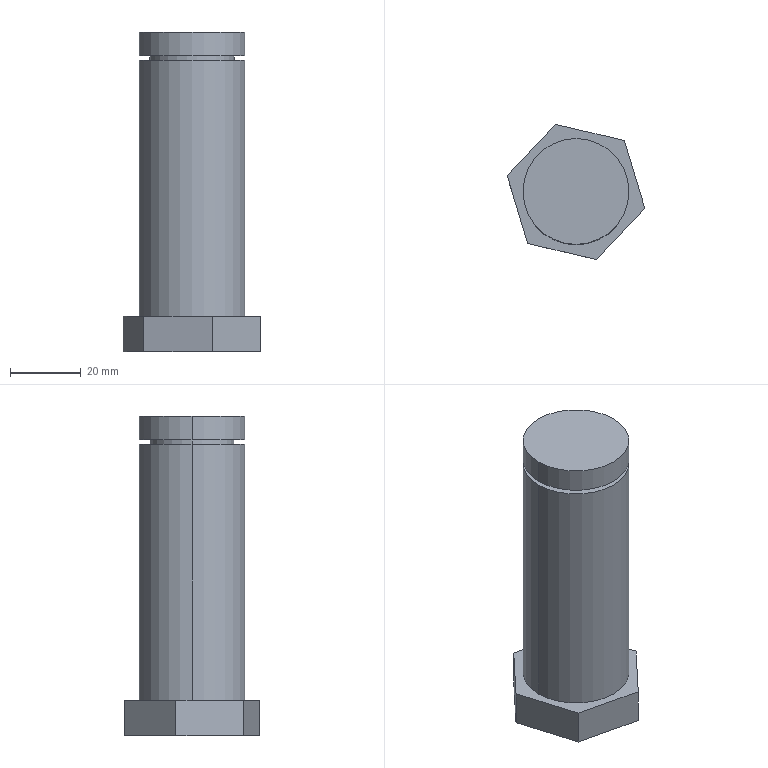Part | STEP file | 1 solid | 17 faces | box 38.947 x 38.288 x 90.5 mm | volume 66959 mm3 | plane 11 | cylinder 6 | commonest cylinder face diameters 30 x4 23.9 x2
STEP:
#1=CARTESIAN_POINT('',(0.,0.,0.));
#2=DIRECTION('',(0.,0.,1.));
#3=DIRECTION('',(1.,0.,0.));
#4=AXIS2_PLACEMENT_3D('',#1,#2,#3);
#5=CARTESIAN_POINT('',(-5.789,19.144,0.));
#6=VERTEX_POINT('',#5);
#7=CARTESIAN_POINT('',(13.684,14.585,0.));
#8=VERTEX_POINT('',#7);
#9=CARTESIAN_POINT('',(-5.789,19.144,0.));
#10=DIRECTION('',(0.9737,-0.2279,0.));
#11=VECTOR('',#10,1.);
#12=LINE('',#9,#11);
#13=CARTESIAN_POINT('',(0.,0.,0.));
#14=DIRECTION('',(0.,0.,1.));
#15=DIRECTION('',(1.,0.,0.));
#16=AXIS2_PLACEMENT_3D('',#13,#14,#15);
#17=PLANE('',#16);
#18=CARTESIAN_POINT('',(-5.789,19.144));
#19=DIRECTION('',(0.9737,-0.2279));
#20=VECTOR('',#19,1.);
#21=LINE('',#18,#20);
#22=(GEOMETRIC_REPRESENTATION_CONTEXT(2)PARAMETRIC_REPRESENTATION_CONTEXT()REPRESENTATION_CONTEXT('',''));
#23=DEFINITIONAL_REPRESENTATION('',(#21),#22);
#24=PCURVE('',#17,#23);
#25=CARTESIAN_POINT('',(-5.789,19.144,80.5));
#26=DIRECTION('',(0.2279,0.9737,0.));
#27=DIRECTION('',(0.,0.,-1.));
#28=AXIS2_PLACEMENT_3D('',#25,#26,#27);
#29=PLANE('',#28);
#30=CARTESIAN_POINT('',(80.5,0.));
#31=DIRECTION('',(0.,-1.));
#32=VECTOR('',#31,1.);
#33=LINE('',#30,#32);
#34=(GEOMETRIC_REPRESENTATION_CONTEXT(2)PARAMETRIC_REPRESENTATION_CONTEXT()REPRESENTATION_CONTEXT('',''));
#35=DEFINITIONAL_REPRESENTATION('',(#33),#34);
#36=PCURVE('',#29,#35);
#37=SURFACE_CURVE('',#12,(#24,#36),.PCURVE_S1.);
#38=EDGE_CURVE('',#6,#8,#37,.T.);
#39=ORIENTED_EDGE('',*,*,#38,.T.);
#40=CARTESIAN_POINT('',(19.474,-4.558,0.));
#41=VERTEX_POINT('',#40);
#42=CARTESIAN_POINT('',(13.684,14.585,0.));
#43=DIRECTION('',(0.2895,-0.9572,0.));
#44=VECTOR('',#43,1.);
#45=LINE('',#42,#44);
#46=CARTESIAN_POINT('',(13.684,14.585));
#47=DIRECTION('',(0.2895,-0.9572));
#48=VECTOR('',#47,1.);
#49=LINE('',#46,#48);
#50=(GEOMETRIC_REPRESENTATION_CONTEXT(2)PARAMETRIC_REPRESENTATION_CONTEXT()REPRESENTATION_CONTEXT('',''));
#51=DEFINITIONAL_REPRESENTATION('',(#49),#50);
#52=PCURVE('',#17,#51);
#53=CARTESIAN_POINT('',(13.684,14.585,80.5));
#54=DIRECTION('',(0.9572,0.2895,0.));
#55=DIRECTION('',(0.,0.,-1.));
#56=AXIS2_PLACEMENT_3D('',#53,#54,#55);
#57=PLANE('',#56);
#58=CARTESIAN_POINT('',(80.5,0.));
#59=DIRECTION('',(0.,-1.));
#60=VECTOR('',#59,1.);
#61=LINE('',#58,#60);
#62=(GEOMETRIC_REPRESENTATION_CONTEXT(2)PARAMETRIC_REPRESENTATION_CONTEXT()REPRESENTATION_CONTEXT('',''));
#63=DEFINITIONAL_REPRESENTATION('',(#61),#62);
#64=PCURVE('',#57,#63);
#65=SURFACE_CURVE('',#45,(#52,#64),.PCURVE_S1.);
#66=EDGE_CURVE('',#8,#41,#65,.T.);
#67=ORIENTED_EDGE('',*,*,#66,.T.);
#68=CARTESIAN_POINT('',(5.789,-19.144,0.));
#69=VERTEX_POINT('',#68);
#70=CARTESIAN_POINT('',(19.474,-4.558,0.));
#71=DIRECTION('',(-0.6842,-0.7293,0.));
#72=VECTOR('',#71,1.);
#73=LINE('',#70,#72);
#74=CARTESIAN_POINT('',(19.474,-4.558));
#75=DIRECTION('',(-0.6842,-0.7293));
#76=VECTOR('',#75,1.);
#77=LINE('',#74,#76);
#78=(GEOMETRIC_REPRESENTATION_CONTEXT(2)PARAMETRIC_REPRESENTATION_CONTEXT()REPRESENTATION_CONTEXT('',''));
#79=DEFINITIONAL_REPRESENTATION('',(#77),#78);
#80=PCURVE('',#17,#79);
#81=CARTESIAN_POINT('',(19.474,-4.558,80.5));
#82=DIRECTION('',(0.7293,-0.6842,0.));
#83=DIRECTION('',(0.,0.,-1.));
#84=AXIS2_PLACEMENT_3D('',#81,#82,#83);
#85=PLANE('',#84);
#86=CARTESIAN_POINT('',(80.5,0.));
#87=DIRECTION('',(0.,-1.));
#88=VECTOR('',#87,1.);
#89=LINE('',#86,#88);
#90=(GEOMETRIC_REPRESENTATION_CONTEXT(2)PARAMETRIC_REPRESENTATION_CONTEXT()REPRESENTATION_CONTEXT('',''));
#91=DEFINITIONAL_REPRESENTATION('',(#89),#90);
#92=PCURVE('',#85,#91);
#93=SURFACE_CURVE('',#73,(#80,#92),.PCURVE_S1.);
#94=EDGE_CURVE('',#41,#69,#93,.T.);
#95=ORIENTED_EDGE('',*,*,#94,.T.);
#96=CARTESIAN_POINT('',(-13.684,-14.585,0.));
#97=VERTEX_POINT('',#96);
#98=CARTESIAN_POINT('',(5.789,-19.144,0.));
#99=DIRECTION('',(-0.9737,0.2279,0.));
#100=VECTOR('',#99,1.);
#101=LINE('',#98,#100);
#102=CARTESIAN_POINT('',(5.789,-19.144));
#103=DIRECTION('',(-0.9737,0.2279));
#104=VECTOR('',#103,1.);
#105=LINE('',#102,#104);
#106=(GEOMETRIC_REPRESENTATION_CONTEXT(2)PARAMETRIC_REPRESENTATION_CONTEXT()REPRESENTATION_CONTEXT('',''));
#107=DEFINITIONAL_REPRESENTATION('',(#105),#106);
#108=PCURVE('',#17,#107);
#109=CARTESIAN_POINT('',(5.789,-19.144,80.5));
#110=DIRECTION('',(-0.2279,-0.9737,0.));
#111=DIRECTION('',(-0.9737,0.2279,0.));
#112=AXIS2_PLACEMENT_3D('',#109,#110,#111);
#113=PLANE('',#112);
#114=CARTESIAN_POINT('',(0.,80.5));
#115=DIRECTION('',(1.,0.));
#116=VECTOR('',#115,1.);
#117=LINE('',#114,#116);
#118=(GEOMETRIC_REPRESENTATION_CONTEXT(2)PARAMETRIC_REPRESENTATION_CONTEXT()REPRESENTATION_CONTEXT('',''));
#119=DEFINITIONAL_REPRESENTATION('',(#117),#118);
#120=PCURVE('',#113,#119);
#121=SURFACE_CURVE('',#101,(#108,#120),.PCURVE_S1.);
#122=EDGE_CURVE('',#69,#97,#121,.T.);
#123=ORIENTED_EDGE('',*,*,#122,.T.);
#124=CARTESIAN_POINT('',(-19.474,4.558,0.));
#125=VERTEX_POINT('',#124);
#126=CARTESIAN_POINT('',(-13.684,-14.585,0.));
#127=DIRECTION('',(-0.2895,0.9572,0.));
#128=VECTOR('',#127,1.);
#129=LINE('',#126,#128);
#130=CARTESIAN_POINT('',(-13.684,-14.585));
#131=DIRECTION('',(-0.2895,0.9572));
#132=VECTOR('',#131,1.);
#133=LINE('',#130,#132);
#134=(GEOMETRIC_REPRESENTATION_CONTEXT(2)PARAMETRIC_REPRESENTATION_CONTEXT()REPRESENTATION_CONTEXT('',''));
#135=DEFINITIONAL_REPRESENTATION('',(#133),#134);
#136=PCURVE('',#17,#135);
#137=CARTESIAN_POINT('',(-13.684,-14.585,80.5));
#138=DIRECTION('',(-0.9572,-0.2895,0.));
#139=DIRECTION('',(-0.2895,0.9572,0.));
#140=AXIS2_PLACEMENT_3D('',#137,#138,#139);
#141=PLANE('',#140);
#142=CARTESIAN_POINT('',(0.,80.5));
#143=DIRECTION('',(1.,0.));
#144=VECTOR('',#143,1.);
#145=LINE('',#142,#144);
#146=(GEOMETRIC_REPRESENTATION_CONTEXT(2)PARAMETRIC_REPRESENTATION_CONTEXT()REPRESENTATION_CONTEXT('',''));
#147=DEFINITIONAL_REPRESENTATION('',(#145),#146);
#148=PCURVE('',#141,#147);
#149=SURFACE_CURVE('',#129,(#136,#148),.PCURVE_S1.);
#150=EDGE_CURVE('',#97,#125,#149,.T.);
#151=ORIENTED_EDGE('',*,*,#150,.T.);
#152=CARTESIAN_POINT('',(-19.474,4.558,0.));
#153=DIRECTION('',(0.6842,0.7293,0.));
#154=VECTOR('',#153,1.);
#155=LINE('',#152,#154);
#156=CARTESIAN_POINT('',(-19.474,4.558));
#157=DIRECTION('',(0.6842,0.7293));
#158=VECTOR('',#157,1.);
#159=LINE('',#156,#158);
#160=(GEOMETRIC_REPRESENTATION_CONTEXT(2)PARAMETRIC_REPRESENTATION_CONTEXT()REPRESENTATION_CONTEXT('',''));
#161=DEFINITIONAL_REPRESENTATION('',(#159),#160);
#162=PCURVE('',#17,#161);
#163=CARTESIAN_POINT('',(-19.474,4.558,80.5));
#164=DIRECTION('',(-0.7293,0.6842,0.));
#165=DIRECTION('',(0.,0.,1.));
#166=AXIS2_PLACEMENT_3D('',#163,#164,#165);
#167=PLANE('',#166);
#168=CARTESIAN_POINT('',(-80.5,0.));
#169=DIRECTION('',(0.,1.));
#170=VECTOR('',#169,1.);
#171=LINE('',#168,#170);
#172=(GEOMETRIC_REPRESENTATION_CONTEXT(2)PARAMETRIC_REPRESENTATION_CONTEXT()REPRESENTATION_CONTEXT('',''));
#173=DEFINITIONAL_REPRESENTATION('',(#171),#172);
#174=PCURVE('',#167,#173);
#175=SURFACE_CURVE('',#155,(#162,#174),.PCURVE_S1.);
#176=EDGE_CURVE('',#125,#6,#175,.T.);
#177=ORIENTED_EDGE('',*,*,#176,.T.);
#178=EDGE_LOOP('',(#39,#67,#95,#123,#151,#177));
#179=FACE_BOUND('',#178,.T.);
#180=ADVANCED_FACE('',(#179),#17,.F.);
#181=CARTESIAN_POINT('',(19.474,-4.558,10.));
#182=VERTEX_POINT('',#181);
#183=CARTESIAN_POINT('',(19.474,-4.558,80.5));
#184=DIRECTION('',(0.,0.,-1.));
#185=VECTOR('',#184,1.);
#186=LINE('',#183,#185);
#187=CARTESIAN_POINT('',(0.,-20.));
#188=DIRECTION('',(1.,0.));
#189=VECTOR('',#188,1.);
#190=LINE('',#187,#189);
#191=(GEOMETRIC_REPRESENTATION_CONTEXT(2)PARAMETRIC_REPRESENTATION_CONTEXT()REPRESENTATION_CONTEXT('',''));
#192=DEFINITIONAL_REPRESENTATION('',(#190),#191);
#193=PCURVE('',#57,#192);
#194=CARTESIAN_POINT('',(0.,0.));
#195=DIRECTION('',(1.,0.));
#196=VECTOR('',#195,1.);
#197=LINE('',#194,#196);
#198=(GEOMETRIC_REPRESENTATION_CONTEXT(2)PARAMETRIC_REPRESENTATION_CONTEXT()REPRESENTATION_CONTEXT('',''));
#199=DEFINITIONAL_REPRESENTATION('',(#197),#198);
#200=PCURVE('',#85,#199);
#201=SURFACE_CURVE('',#186,(#193,#200),.PCURVE_S1.);
#202=EDGE_CURVE('',#182,#41,#201,.T.);
#203=ORIENTED_EDGE('',*,*,#202,.T.);
#204=ORIENTED_EDGE('',*,*,#66,.F.);
#205=CARTESIAN_POINT('',(13.684,14.585,10.));
#206=VERTEX_POINT('',#205);
#207=CARTESIAN_POINT('',(13.684,14.585,80.5));
#208=DIRECTION('',(0.,0.,-1.));
#209=VECTOR('',#208,1.);
#210=LINE('',#207,#209);
#211=CARTESIAN_POINT('',(0.,0.));
#212=DIRECTION('',(1.,0.));
#213=VECTOR('',#212,1.);
#214=LINE('',#211,#213);
#215=(GEOMETRIC_REPRESENTATION_CONTEXT(2)PARAMETRIC_REPRESENTATION_CONTEXT()REPRESENTATION_CONTEXT('',''));
#216=DEFINITIONAL_REPRESENTATION('',(#214),#215);
#217=PCURVE('',#57,#216);
#218=CARTESIAN_POINT('',(0.,-20.));
#219=DIRECTION('',(1.,0.));
#220=VECTOR('',#219,1.);
#221=LINE('',#218,#220);
#222=(GEOMETRIC_REPRESENTATION_CONTEXT(2)PARAMETRIC_REPRESENTATION_CONTEXT()REPRESENTATION_CONTEXT('',''));
#223=DEFINITIONAL_REPRESENTATION('',(#221),#222);
#224=PCURVE('',#29,#223);
#225=SURFACE_CURVE('',#210,(#217,#224),.PCURVE_S1.);
#226=EDGE_CURVE('',#206,#8,#225,.T.);
#227=ORIENTED_EDGE('',*,*,#226,.F.);
#228=CARTESIAN_POINT('',(16.579,5.014,10.));
#229=DIRECTION('',(-0.2895,0.9572,0.));
#230=VECTOR('',#229,1.);
#231=LINE('',#228,#230);
#232=CARTESIAN_POINT('',(70.5,-10.));
#233=DIRECTION('',(0.,1.));
#234=VECTOR('',#233,1.);
#235=LINE('',#232,#234);
#236=(GEOMETRIC_REPRESENTATION_CONTEXT(2)PARAMETRIC_REPRESENTATION_CONTEXT()REPRESENTATION_CONTEXT('',''));
#237=DEFINITIONAL_REPRESENTATION('',(#235),#236);
#238=PCURVE('',#57,#237);
#239=CARTESIAN_POINT('',(0.,0.,10.));
#240=DIRECTION('',(0.,0.,1.));
#241=DIRECTION('',(1.,0.,0.));
#242=AXIS2_PLACEMENT_3D('',#239,#240,#241);
#243=PLANE('',#242);
#244=CARTESIAN_POINT('',(16.579,5.014));
#245=DIRECTION('',(-0.2895,0.9572));
#246=VECTOR('',#245,1.);
#247=LINE('',#244,#246);
#248=(GEOMETRIC_REPRESENTATION_CONTEXT(2)PARAMETRIC_REPRESENTATION_CONTEXT()REPRESENTATION_CONTEXT('',''));
#249=DEFINITIONAL_REPRESENTATION('',(#247),#248);
#250=PCURVE('',#243,#249);
#251=SURFACE_CURVE('',#231,(#238,#250),.PCURVE_S1.);
#252=EDGE_CURVE('',#182,#206,#251,.T.);
#253=ORIENTED_EDGE('',*,*,#252,.F.);
#254=EDGE_LOOP('',(#203,#204,#227,#253));
#255=FACE_BOUND('',#254,.T.);
#256=ADVANCED_FACE('',(#255),#57,.T.);
#257=CARTESIAN_POINT('',(5.789,-19.144,10.));
#258=VERTEX_POINT('',#257);
#259=CARTESIAN_POINT('',(5.789,-19.144,80.5));
#260=DIRECTION('',(0.,0.,-1.));
#261=VECTOR('',#260,1.);
#262=LINE('',#259,#261);
#263=CARTESIAN_POINT('',(0.,-20.));
#264=DIRECTION('',(1.,0.));
#265=VECTOR('',#264,1.);
#266=LINE('',#263,#265);
#267=(GEOMETRIC_REPRESENTATION_CONTEXT(2)PARAMETRIC_REPRESENTATION_CONTEXT()REPRESENTATION_CONTEXT('',''));
#268=DEFINITIONAL_REPRESENTATION('',(#266),#267);
#269=PCURVE('',#85,#268);
#270=CARTESIAN_POINT('',(0.,0.));
#271=DIRECTION('',(0.,1.));
#272=VECTOR('',#271,1.);
#273=LINE('',#270,#272);
#274=(GEOMETRIC_REPRESENTATION_CONTEXT(2)PARAMETRIC_REPRESENTATION_CONTEXT()REPRESENTATION_CONTEXT('',''));
#275=DEFINITIONAL_REPRESENTATION('',(#273),#274);
#276=PCURVE('',#113,#275);
#277=SURFACE_CURVE('',#262,(#269,#276),.PCURVE_S1.);
#278=EDGE_CURVE('',#258,#69,#277,.T.);
#279=ORIENTED_EDGE('',*,*,#278,.T.);
#280=ORIENTED_EDGE('',*,*,#94,.F.);
#281=ORIENTED_EDGE('',*,*,#202,.F.);
#282=CARTESIAN_POINT('',(12.631,-11.851,10.));
#283=DIRECTION('',(0.6842,0.7293,0.));
#284=VECTOR('',#283,1.);
#285=LINE('',#282,#284);
#286=CARTESIAN_POINT('',(70.5,-10.));
#287=DIRECTION('',(0.,1.));
#288=VECTOR('',#287,1.);
#289=LINE('',#286,#288);
#290=(GEOMETRIC_REPRESENTATION_CONTEXT(2)PARAMETRIC_REPRESENTATION_CONTEXT()REPRESENTATION_CONTEXT('',''));
#291=DEFINITIONAL_REPRESENTATION('',(#289),#290);
#292=PCURVE('',#85,#291);
#293=CARTESIAN_POINT('',(12.631,-11.851));
#294=DIRECTION('',(0.6842,0.7293));
#295=VECTOR('',#294,1.);
#296=LINE('',#293,#295);
#297=(GEOMETRIC_REPRESENTATION_CONTEXT(2)PARAMETRIC_REPRESENTATION_CONTEXT()REPRESENTATION_CONTEXT('',''));
#298=DEFINITIONAL_REPRESENTATION('',(#296),#297);
#299=PCURVE('',#243,#298);
#300=SURFACE_CURVE('',#285,(#292,#299),.PCURVE_S1.);
#301=EDGE_CURVE('',#258,#182,#300,.T.);
#302=ORIENTED_EDGE('',*,*,#301,.F.);
#303=EDGE_LOOP('',(#279,#280,#281,#302));
#304=FACE_BOUND('',#303,.T.);
#305=ADVANCED_FACE('',(#304),#85,.T.);
#306=CARTESIAN_POINT('',(-13.684,-14.585,10.));
#307=VERTEX_POINT('',#306);
#308=CARTESIAN_POINT('',(-13.684,-14.585,80.5));
#309=DIRECTION('',(0.,0.,-1.));
#310=VECTOR('',#309,1.);
#311=LINE('',#308,#310);
#312=CARTESIAN_POINT('',(20.,0.));
#313=DIRECTION('',(0.,1.));
#314=VECTOR('',#313,1.);
#315=LINE('',#312,#314);
#316=(GEOMETRIC_REPRESENTATION_CONTEXT(2)PARAMETRIC_REPRESENTATION_CONTEXT()REPRESENTATION_CONTEXT('',''));
#317=DEFINITIONAL_REPRESENTATION('',(#315),#316);
#318=PCURVE('',#113,#317);
#319=CARTESIAN_POINT('',(0.,0.));
#320=DIRECTION('',(0.,1.));
#321=VECTOR('',#320,1.);
#322=LINE('',#319,#321);
#323=(GEOMETRIC_REPRESENTATION_CONTEXT(2)PARAMETRIC_REPRESENTATION_CONTEXT()REPRESENTATION_CONTEXT('',''));
#324=DEFINITIONAL_REPRESENTATION('',(#322),#323);
#325=PCURVE('',#141,#324);
#326=SURFACE_CURVE('',#311,(#318,#325),.PCURVE_S1.);
#327=EDGE_CURVE('',#307,#97,#326,.T.);
#328=ORIENTED_EDGE('',*,*,#327,.T.);
#329=ORIENTED_EDGE('',*,*,#122,.F.);
#330=ORIENTED_EDGE('',*,*,#278,.F.);
#331=CARTESIAN_POINT('',(-3.948,-16.865,10.));
#332=DIRECTION('',(0.9737,-0.2279,0.));
#333=VECTOR('',#332,1.);
#334=LINE('',#331,#333);
#335=CARTESIAN_POINT('',(10.,70.5));
#336=DIRECTION('',(-1.,0.));
#337=VECTOR('',#336,1.);
#338=LINE('',#335,#337);
#339=(GEOMETRIC_REPRESENTATION_CONTEXT(2)PARAMETRIC_REPRESENTATION_CONTEXT()REPRESENTATION_CONTEXT('',''));
#340=DEFINITIONAL_REPRESENTATION('',(#338),#339);
#341=PCURVE('',#113,#340);
#342=CARTESIAN_POINT('',(-3.948,-16.865));
#343=DIRECTION('',(0.9737,-0.2279));
#344=VECTOR('',#343,1.);
#345=LINE('',#342,#344);
#346=(GEOMETRIC_REPRESENTATION_CONTEXT(2)PARAMETRIC_REPRESENTATION_CONTEXT()REPRESENTATION_CONTEXT('',''));
#347=DEFINITIONAL_REPRESENTATION('',(#345),#346);
#348=PCURVE('',#243,#347);
#349=SURFACE_CURVE('',#334,(#341,#348),.PCURVE_S1.);
#350=EDGE_CURVE('',#307,#258,#349,.T.);
#351=ORIENTED_EDGE('',*,*,#350,.F.);
#352=EDGE_LOOP('',(#328,#329,#330,#351));
#353=FACE_BOUND('',#352,.T.);
#354=ADVANCED_FACE('',(#353),#113,.T.);
#355=CARTESIAN_POINT('',(-19.474,4.558,10.));
#356=VERTEX_POINT('',#355);
#357=CARTESIAN_POINT('',(-19.474,4.558,80.5));
#358=DIRECTION('',(0.,0.,-1.));
#359=VECTOR('',#358,1.);
#360=LINE('',#357,#359);
#361=CARTESIAN_POINT('',(20.,0.));
#362=DIRECTION('',(0.,1.));
#363=VECTOR('',#362,1.);
#364=LINE('',#361,#363);
#365=(GEOMETRIC_REPRESENTATION_CONTEXT(2)PARAMETRIC_REPRESENTATION_CONTEXT()REPRESENTATION_CONTEXT('',''));
#366=DEFINITIONAL_REPRESENTATION('',(#364),#365);
#367=PCURVE('',#141,#366);
#368=CARTESIAN_POINT('',(0.,0.));
#369=DIRECTION('',(-1.,0.));
#370=VECTOR('',#369,1.);
#371=LINE('',#368,#370);
#372=(GEOMETRIC_REPRESENTATION_CONTEXT(2)PARAMETRIC_REPRESENTATION_CONTEXT()REPRESENTATION_CONTEXT('',''));
#373=DEFINITIONAL_REPRESENTATION('',(#371),#372);
#374=PCURVE('',#167,#373);
#375=SURFACE_CURVE('',#360,(#367,#374),.PCURVE_S1.);
#376=EDGE_CURVE('',#356,#125,#375,.T.);
#377=ORIENTED_EDGE('',*,*,#376,.T.);
#378=ORIENTED_EDGE('',*,*,#150,.F.);
#379=ORIENTED_EDGE('',*,*,#327,.F.);
#380=CARTESIAN_POINT('',(-16.579,-5.014,10.));
#381=DIRECTION('',(0.2895,-0.9572,0.));
#382=VECTOR('',#381,1.);
#383=LINE('',#380,#382);
#384=CARTESIAN_POINT('',(10.,70.5));
#385=DIRECTION('',(-1.,0.));
#386=VECTOR('',#385,1.);
#387=LINE('',#384,#386);
#388=(GEOMETRIC_REPRESENTATION_CONTEXT(2)PARAMETRIC_REPRESENTATION_CONTEXT()REPRESENTATION_CONTEXT('',''));
#389=DEFINITIONAL_REPRESENTATION('',(#387),#388);
#390=PCURVE('',#141,#389);
#391=CARTESIAN_POINT('',(-16.579,-5.014));
#392=DIRECTION('',(0.2895,-0.9572));
#393=VECTOR('',#392,1.);
#394=LINE('',#391,#393);
#395=(GEOMETRIC_REPRESENTATION_CONTEXT(2)PARAMETRIC_REPRESENTATION_CONTEXT()REPRESENTATION_CONTEXT('',''));
#396=DEFINITIONAL_REPRESENTATION('',(#394),#395);
#397=PCURVE('',#243,#396);
#398=SURFACE_CURVE('',#383,(#390,#397),.PCURVE_S1.);
#399=EDGE_CURVE('',#356,#307,#398,.T.);
#400=ORIENTED_EDGE('',*,*,#399,.F.);
#401=EDGE_LOOP('',(#377,#378,#379,#400));
#402=FACE_BOUND('',#401,.T.);
#403=ADVANCED_FACE('',(#402),#141,.T.);
#404=CARTESIAN_POINT('',(-5.789,19.144,10.));
#405=VERTEX_POINT('',#404);
#406=CARTESIAN_POINT('',(-5.789,19.144,80.5));
#407=DIRECTION('',(0.,0.,-1.));
#408=VECTOR('',#407,1.);
#409=LINE('',#406,#408);
#410=CARTESIAN_POINT('',(0.,20.));
#411=DIRECTION('',(-1.,0.));
#412=VECTOR('',#411,1.);
#413=LINE('',#410,#412);
#414=(GEOMETRIC_REPRESENTATION_CONTEXT(2)PARAMETRIC_REPRESENTATION_CONTEXT()REPRESENTATION_CONTEXT('',''));
#415=DEFINITIONAL_REPRESENTATION('',(#413),#414);
#416=PCURVE('',#167,#415);
#417=CARTESIAN_POINT('',(0.,0.));
#418=DIRECTION('',(1.,0.));
#419=VECTOR('',#418,1.);
#420=LINE('',#417,#419);
#421=(GEOMETRIC_REPRESENTATION_CONTEXT(2)PARAMETRIC_REPRESENTATION_CONTEXT()REPRESENTATION_CONTEXT('',''));
#422=DEFINITIONAL_REPRESENTATION('',(#420),#421);
#423=PCURVE('',#29,#422);
#424=SURFACE_CURVE('',#409,(#416,#423),.PCURVE_S1.);
#425=EDGE_CURVE('',#405,#6,#424,.T.);
#426=ORIENTED_EDGE('',*,*,#425,.T.);
#427=ORIENTED_EDGE('',*,*,#176,.F.);
#428=ORIENTED_EDGE('',*,*,#376,.F.);
#429=CARTESIAN_POINT('',(-12.631,11.851,10.));
#430=DIRECTION('',(-0.6842,-0.7293,0.));
#431=VECTOR('',#430,1.);
#432=LINE('',#429,#431);
#433=CARTESIAN_POINT('',(-70.5,10.));
#434=DIRECTION('',(0.,-1.));
#435=VECTOR('',#434,1.);
#436=LINE('',#433,#435);
#437=(GEOMETRIC_REPRESENTATION_CONTEXT(2)PARAMETRIC_REPRESENTATION_CONTEXT()REPRESENTATION_CONTEXT('',''));
#438=DEFINITIONAL_REPRESENTATION('',(#436),#437);
#439=PCURVE('',#167,#438);
#440=CARTESIAN_POINT('',(-12.631,11.851));
#441=DIRECTION('',(-0.6842,-0.7293));
#442=VECTOR('',#441,1.);
#443=LINE('',#440,#442);
#444=(GEOMETRIC_REPRESENTATION_CONTEXT(2)PARAMETRIC_REPRESENTATION_CONTEXT()REPRESENTATION_CONTEXT('',''));
#445=DEFINITIONAL_REPRESENTATION('',(#443),#444);
#446=PCURVE('',#243,#445);
#447=SURFACE_CURVE('',#432,(#439,#446),.PCURVE_S1.);
#448=EDGE_CURVE('',#405,#356,#447,.T.);
#449=ORIENTED_EDGE('',*,*,#448,.F.);
#450=EDGE_LOOP('',(#426,#427,#428,#449));
#451=FACE_BOUND('',#450,.T.);
#452=ADVANCED_FACE('',(#451),#167,.T.);
#453=ORIENTED_EDGE('',*,*,#226,.T.);
#454=ORIENTED_EDGE('',*,*,#38,.F.);
#455=ORIENTED_EDGE('',*,*,#425,.F.);
#456=CARTESIAN_POINT('',(3.948,16.865,10.));
#457=DIRECTION('',(-0.9737,0.2279,0.));
#458=VECTOR('',#457,1.);
#459=LINE('',#456,#458);
#460=CARTESIAN_POINT('',(70.5,-10.));
#461=DIRECTION('',(0.,1.));
#462=VECTOR('',#461,1.);
#463=LINE('',#460,#462);
#464=(GEOMETRIC_REPRESENTATION_CONTEXT(2)PARAMETRIC_REPRESENTATION_CONTEXT()REPRESENTATION_CONTEXT('',''));
#465=DEFINITIONAL_REPRESENTATION('',(#463),#464);
#466=PCURVE('',#29,#465);
#467=CARTESIAN_POINT('',(3.948,16.865));
#468=DIRECTION('',(-0.9737,0.2279));
#469=VECTOR('',#468,1.);
#470=LINE('',#467,#469);
#471=(GEOMETRIC_REPRESENTATION_CONTEXT(2)PARAMETRIC_REPRESENTATION_CONTEXT()REPRESENTATION_CONTEXT('',''));
#472=DEFINITIONAL_REPRESENTATION('',(#470),#471);
#473=PCURVE('',#243,#472);
#474=SURFACE_CURVE('',#459,(#466,#473),.PCURVE_S1.);
#475=EDGE_CURVE('',#206,#405,#474,.T.);
#476=ORIENTED_EDGE('',*,*,#475,.F.);
#477=EDGE_LOOP('',(#453,#454,#455,#476));
#478=FACE_BOUND('',#477,.T.);
#479=ADVANCED_FACE('',(#478),#29,.T.);
#480=CARTESIAN_POINT('',(15.,0.,90.5));
#481=VERTEX_POINT('',#480);
#482=CARTESIAN_POINT('',(15.,0.,83.8));
#483=VERTEX_POINT('',#482);
#484=CARTESIAN_POINT('',(15.,0.,90.5));
#485=DIRECTION('',(0.,0.,-1.));
#486=VECTOR('',#485,1.);
#487=LINE('',#484,#486);
#488=CARTESIAN_POINT('',(0.,0.,90.5));
#489=DIRECTION('',(0.,0.,-1.));
#490=DIRECTION('',(-1.,0.,0.));
#491=AXIS2_PLACEMENT_3D('',#488,#489,#490);
#492=CYLINDRICAL_SURFACE('',#491,15.);
#493=CARTESIAN_POINT('',(3.142,0.));
#494=DIRECTION('',(0.,1.));
#495=VECTOR('',#494,1.);
#496=LINE('',#493,#495);
#497=(GEOMETRIC_REPRESENTATION_CONTEXT(2)PARAMETRIC_REPRESENTATION_CONTEXT()REPRESENTATION_CONTEXT('',''));
#498=DEFINITIONAL_REPRESENTATION('',(#496),#497);
#499=PCURVE('',#492,#498);
#500=CARTESIAN_POINT('',(0.,0.,90.5));
#501=DIRECTION('',(0.,0.,-1.));
#502=DIRECTION('',(-1.,0.,0.));
#503=AXIS2_PLACEMENT_3D('',#500,#501,#502);
#504=CYLINDRICAL_SURFACE('',#503,15.);
#505=CARTESIAN_POINT('',(3.142,0.));
#506=DIRECTION('',(0.,1.));
#507=VECTOR('',#506,1.);
#508=LINE('',#505,#507);
#509=(GEOMETRIC_REPRESENTATION_CONTEXT(2)PARAMETRIC_REPRESENTATION_CONTEXT()REPRESENTATION_CONTEXT('',''));
#510=DEFINITIONAL_REPRESENTATION('',(#508),#509);
#511=PCURVE('',#504,#510);
#512=SURFACE_CURVE('',#487,(#499,#511),.PCURVE_S1.);
#513=EDGE_CURVE('',#481,#483,#512,.T.);
#514=ORIENTED_EDGE('',*,*,#513,.F.);
#515=CARTESIAN_POINT('',(-15.,0.,90.5));
#516=VERTEX_POINT('',#515);
#517=CARTESIAN_POINT('',(0.,0.,90.5));
#518=DIRECTION('',(0.,0.,1.));
#519=DIRECTION('',(1.,0.,0.));
#520=AXIS2_PLACEMENT_3D('',#517,#518,#519);
#521=CIRCLE('',#520,15.);
#522=CARTESIAN_POINT('',(9.425,0.));
#523=DIRECTION('',(-1.,0.));
#524=VECTOR('',#523,1.);
#525=LINE('',#522,#524);
#526=(GEOMETRIC_REPRESENTATION_CONTEXT(2)PARAMETRIC_REPRESENTATION_CONTEXT()REPRESENTATION_CONTEXT('',''));
#527=DEFINITIONAL_REPRESENTATION('',(#525),#526);
#528=PCURVE('',#492,#527);
#529=CARTESIAN_POINT('',(0.,0.,90.5));
#530=DIRECTION('',(0.,0.,1.));
#531=DIRECTION('',(1.,0.,0.));
#532=AXIS2_PLACEMENT_3D('',#529,#530,#531);
#533=PLANE('',#532);
#534=CARTESIAN_POINT('',(0.,0.));
#535=DIRECTION('',(1.,0.));
#536=AXIS2_PLACEMENT_2D('',#534,#535);
#537=CIRCLE('',#536,15.);
#538=(GEOMETRIC_REPRESENTATION_CONTEXT(2)PARAMETRIC_REPRESENTATION_CONTEXT()REPRESENTATION_CONTEXT('',''));
#539=DEFINITIONAL_REPRESENTATION('',(#537),#538);
#540=PCURVE('',#533,#539);
#541=SURFACE_CURVE('',#521,(#528,#540),.PCURVE_S1.);
#542=EDGE_CURVE('',#516,#481,#541,.T.);
#543=ORIENTED_EDGE('',*,*,#542,.F.);
#544=CARTESIAN_POINT('',(-15.,0.,83.8));
#545=VERTEX_POINT('',#544);
#546=CARTESIAN_POINT('',(-15.,0.,90.5));
#547=DIRECTION('',(0.,0.,-1.));
#548=VECTOR('',#547,1.);
#549=LINE('',#546,#548);
#550=CARTESIAN_POINT('',(6.283,0.));
#551=DIRECTION('',(0.,1.));
#552=VECTOR('',#551,1.);
#553=LINE('',#550,#552);
#554=(GEOMETRIC_REPRESENTATION_CONTEXT(2)PARAMETRIC_REPRESENTATION_CONTEXT()REPRESENTATION_CONTEXT('',''));
#555=DEFINITIONAL_REPRESENTATION('',(#553),#554);
#556=PCURVE('',#492,#555);
#557=CARTESIAN_POINT('',(0.,0.));
#558=DIRECTION('',(0.,1.));
#559=VECTOR('',#558,1.);
#560=LINE('',#557,#559);
#561=(GEOMETRIC_REPRESENTATION_CONTEXT(2)PARAMETRIC_REPRESENTATION_CONTEXT()REPRESENTATION_CONTEXT('',''));
#562=DEFINITIONAL_REPRESENTATION('',(#560),#561);
#563=PCURVE('',#504,#562);
#564=SURFACE_CURVE('',#549,(#556,#563),.PCURVE_S1.);
#565=EDGE_CURVE('',#516,#545,#564,.T.);
#566=ORIENTED_EDGE('',*,*,#565,.T.);
#567=CARTESIAN_POINT('',(0.,0.,83.8));
#568=DIRECTION('',(0.,0.,-1.));
#569=DIRECTION('',(-1.,0.,0.));
#570=AXIS2_PLACEMENT_3D('',#567,#568,#569);
#571=CIRCLE('',#570,15.);
#572=CARTESIAN_POINT('',(0.,6.7));
#573=DIRECTION('',(1.,0.));
#574=VECTOR('',#573,1.);
#575=LINE('',#572,#574);
#576=(GEOMETRIC_REPRESENTATION_CONTEXT(2)PARAMETRIC_REPRESENTATION_CONTEXT()REPRESENTATION_CONTEXT('',''));
#577=DEFINITIONAL_REPRESENTATION('',(#575),#576);
#578=PCURVE('',#492,#577);
#579=CARTESIAN_POINT('',(-17.06,0.,83.8));
#580=DIRECTION('',(0.,0.,-1.));
#581=DIRECTION('',(0.,-1.,0.));
#582=AXIS2_PLACEMENT_3D('',#579,#580,#581);
#583=PLANE('',#582);
#584=CARTESIAN_POINT('',(0.,-17.06));
#585=DIRECTION('',(0.,1.));
#586=AXIS2_PLACEMENT_2D('',#584,#585);
#587=CIRCLE('',#586,15.);
#588=(GEOMETRIC_REPRESENTATION_CONTEXT(2)PARAMETRIC_REPRESENTATION_CONTEXT()REPRESENTATION_CONTEXT('',''));
#589=DEFINITIONAL_REPRESENTATION('',(#587),#588);
#590=PCURVE('',#583,#589);
#591=SURFACE_CURVE('',#571,(#578,#590),.PCURVE_S1.);
#592=EDGE_CURVE('',#483,#545,#591,.T.);
#593=ORIENTED_EDGE('',*,*,#592,.F.);
#594=EDGE_LOOP('',(#514,#543,#566,#593));
#595=FACE_BOUND('',#594,.T.);
#596=ADVANCED_FACE('',(#595),#492,.T.);
#597=ORIENTED_EDGE('',*,*,#542,.T.);
#598=CARTESIAN_POINT('',(0.,0.,90.5));
#599=DIRECTION('',(0.,0.,1.));
#600=DIRECTION('',(1.,0.,0.));
#601=AXIS2_PLACEMENT_3D('',#598,#599,#600);
#602=CIRCLE('',#601,15.);
#603=CARTESIAN_POINT('',(0.,0.));
#604=DIRECTION('',(1.,0.));
#605=AXIS2_PLACEMENT_2D('',#603,#604);
#606=CIRCLE('',#605,15.);
#607=(GEOMETRIC_REPRESENTATION_CONTEXT(2)PARAMETRIC_REPRESENTATION_CONTEXT()REPRESENTATION_CONTEXT('',''));
#608=DEFINITIONAL_REPRESENTATION('',(#606),#607);
#609=PCURVE('',#533,#608);
#610=CARTESIAN_POINT('',(3.142,0.));
#611=DIRECTION('',(-1.,0.));
#612=VECTOR('',#611,1.);
#613=LINE('',#610,#612);
#614=(GEOMETRIC_REPRESENTATION_CONTEXT(2)PARAMETRIC_REPRESENTATION_CONTEXT()REPRESENTATION_CONTEXT('',''));
#615=DEFINITIONAL_REPRESENTATION('',(#613),#614);
#616=PCURVE('',#504,#615);
#617=SURFACE_CURVE('',#602,(#609,#616),.PCURVE_S1.);
#618=EDGE_CURVE('',#481,#516,#617,.T.);
#619=ORIENTED_EDGE('',*,*,#618,.T.);
#620=EDGE_LOOP('',(#597,#619));
#621=FACE_BOUND('',#620,.T.);
#622=ADVANCED_FACE('',(#621),#533,.T.);
#623=CARTESIAN_POINT('',(-11.95,0.,82.5));
#624=VERTEX_POINT('',#623);
#625=CARTESIAN_POINT('',(-11.95,0.,83.8));
#626=VERTEX_POINT('',#625);
#627=CARTESIAN_POINT('',(-11.95,0.,94.725));
#628=DIRECTION('',(0.,0.,1.));
#629=VECTOR('',#628,1.);
#630=LINE('',#627,#629);
#631=CARTESIAN_POINT('',(0.,0.,94.725));
#632=DIRECTION('',(0.,0.,1.));
#633=DIRECTION('',(1.,0.,0.));
#634=AXIS2_PLACEMENT_3D('',#631,#632,#633);
#635=CYLINDRICAL_SURFACE('',#634,11.95);
#636=CARTESIAN_POINT('',(3.142,0.));
#637=DIRECTION('',(0.,1.));
#638=VECTOR('',#637,1.);
#639=LINE('',#636,#638);
#640=(GEOMETRIC_REPRESENTATION_CONTEXT(2)PARAMETRIC_REPRESENTATION_CONTEXT()REPRESENTATION_CONTEXT('',''));
#641=DEFINITIONAL_REPRESENTATION('',(#639),#640);
#642=PCURVE('',#635,#641);
#643=CARTESIAN_POINT('',(0.,0.,94.725));
#644=DIRECTION('',(0.,0.,1.));
#645=DIRECTION('',(1.,0.,0.));
#646=AXIS2_PLACEMENT_3D('',#643,#644,#645);
#647=CYLINDRICAL_SURFACE('',#646,11.95);
#648=CARTESIAN_POINT('',(3.142,0.));
#649=DIRECTION('',(0.,1.));
#650=VECTOR('',#649,1.);
#651=LINE('',#648,#650);
#652=(GEOMETRIC_REPRESENTATION_CONTEXT(2)PARAMETRIC_REPRESENTATION_CONTEXT()REPRESENTATION_CONTEXT('',''));
#653=DEFINITIONAL_REPRESENTATION('',(#651),#652);
#654=PCURVE('',#647,#653);
#655=SURFACE_CURVE('',#630,(#642,#654),.PCURVE_S1.);
#656=EDGE_CURVE('',#624,#626,#655,.T.);
#657=ORIENTED_EDGE('',*,*,#656,.F.);
#658=CARTESIAN_POINT('',(11.95,0.,82.5));
#659=VERTEX_POINT('',#658);
#660=CARTESIAN_POINT('',(0.,0.,82.5));
#661=DIRECTION('',(0.,0.,1.));
#662=DIRECTION('',(1.,0.,0.));
#663=AXIS2_PLACEMENT_3D('',#660,#661,#662);
#664=CIRCLE('',#663,11.95);
#665=CARTESIAN_POINT('',(0.,-12.225));
#666=DIRECTION('',(1.,0.));
#667=VECTOR('',#666,1.);
#668=LINE('',#665,#667);
#669=(GEOMETRIC_REPRESENTATION_CONTEXT(2)PARAMETRIC_REPRESENTATION_CONTEXT()REPRESENTATION_CONTEXT('',''));
#670=DEFINITIONAL_REPRESENTATION('',(#668),#669);
#671=PCURVE('',#635,#670);
#672=CARTESIAN_POINT('',(-17.06,0.,82.5));
#673=DIRECTION('',(0.,0.,1.));
#674=DIRECTION('',(1.,0.,0.));
#675=AXIS2_PLACEMENT_3D('',#672,#673,#674);
#676=PLANE('',#675);
#677=CARTESIAN_POINT('',(17.06,0.));
#678=DIRECTION('',(1.,0.));
#679=AXIS2_PLACEMENT_2D('',#677,#678);
#680=CIRCLE('',#679,11.95);
#681=(GEOMETRIC_REPRESENTATION_CONTEXT(2)PARAMETRIC_REPRESENTATION_CONTEXT()REPRESENTATION_CONTEXT('',''));
#682=DEFINITIONAL_REPRESENTATION('',(#680),#681);
#683=PCURVE('',#676,#682);
#684=SURFACE_CURVE('',#664,(#671,#683),.PCURVE_S1.);
#685=EDGE_CURVE('',#624,#659,#684,.T.);
#686=ORIENTED_EDGE('',*,*,#685,.T.);
#687=CARTESIAN_POINT('',(11.95,0.,83.8));
#688=VERTEX_POINT('',#687);
#689=CARTESIAN_POINT('',(11.95,0.,94.725));
#690=DIRECTION('',(0.,0.,1.));
#691=VECTOR('',#690,1.);
#692=LINE('',#689,#691);
#693=CARTESIAN_POINT('',(6.283,0.));
#694=DIRECTION('',(0.,1.));
#695=VECTOR('',#694,1.);
#696=LINE('',#693,#695);
#697=(GEOMETRIC_REPRESENTATION_CONTEXT(2)PARAMETRIC_REPRESENTATION_CONTEXT()REPRESENTATION_CONTEXT('',''));
#698=DEFINITIONAL_REPRESENTATION('',(#696),#697);
#699=PCURVE('',#635,#698);
#700=CARTESIAN_POINT('',(0.,0.));
#701=DIRECTION('',(0.,1.));
#702=VECTOR('',#701,1.);
#703=LINE('',#700,#702);
#704=(GEOMETRIC_REPRESENTATION_CONTEXT(2)PARAMETRIC_REPRESENTATION_CONTEXT()REPRESENTATION_CONTEXT('',''));
#705=DEFINITIONAL_REPRESENTATION('',(#703),#704);
#706=PCURVE('',#647,#705);
#707=SURFACE_CURVE('',#692,(#699,#706),.PCURVE_S1.);
#708=EDGE_CURVE('',#659,#688,#707,.T.);
#709=ORIENTED_EDGE('',*,*,#708,.T.);
#710=CARTESIAN_POINT('',(0.,0.,83.8));
#711=DIRECTION('',(0.,0.,1.));
#712=DIRECTION('',(1.,0.,0.));
#713=AXIS2_PLACEMENT_3D('',#710,#711,#712);
#714=CIRCLE('',#713,11.95);
#715=CARTESIAN_POINT('',(0.,-10.925));
#716=DIRECTION('',(1.,0.));
#717=VECTOR('',#716,1.);
#718=LINE('',#715,#717);
#719=(GEOMETRIC_REPRESENTATION_CONTEXT(2)PARAMETRIC_REPRESENTATION_CONTEXT()REPRESENTATION_CONTEXT('',''));
#720=DEFINITIONAL_REPRESENTATION('',(#718),#719);
#721=PCURVE('',#635,#720);
#722=CARTESIAN_POINT('',(0.,-29.01));
#723=CARTESIAN_POINT('',(-20.698,-29.01));
#724=CARTESIAN_POINT('',(-10.349,-11.085));
#725=CARTESIAN_POINT('',(0.,6.84));
#726=CARTESIAN_POINT('',(10.349,-11.085));
#727=CARTESIAN_POINT('',(20.698,-29.01));
#728=CARTESIAN_POINT('',(0.,-29.01));
#729=(BOUNDED_CURVE()B_SPLINE_CURVE(2,(#722,#723,#724,#725,#726,#727,#728),.UNSPECIFIED.,.T.,.F.)B_SPLINE_CURVE_WITH_KNOTS((1,2,2,2,2,1),(-2.094,0.,2.094,4.189,6.283,8.378),.UNSPECIFIED.)CURVE()GEOMETRIC_REPRESENTATION_ITEM()RATIONAL_B_SPLINE_CURVE((1.,0.5,1.,0.5,1.,0.5,1.))REPRESENTATION_ITEM(''));
#730=(GEOMETRIC_REPRESENTATION_CONTEXT(2)PARAMETRIC_REPRESENTATION_CONTEXT()REPRESENTATION_CONTEXT('',''));
#731=DEFINITIONAL_REPRESENTATION('',(#729),#730);
#732=PCURVE('',#583,#731);
#733=SURFACE_CURVE('',#714,(#721,#732),.PCURVE_S1.);
#734=EDGE_CURVE('',#626,#688,#733,.T.);
#735=ORIENTED_EDGE('',*,*,#734,.F.);
#736=EDGE_LOOP('',(#657,#686,#709,#735));
#737=FACE_BOUND('',#736,.T.);
#738=ADVANCED_FACE('',(#737),#635,.T.);
#739=CARTESIAN_POINT('',(0.,0.,82.5));
#740=DIRECTION('',(0.,0.,1.));
#741=DIRECTION('',(1.,0.,0.));
#742=AXIS2_PLACEMENT_3D('',#739,#740,#741);
#743=CIRCLE('',#742,11.95);
#744=CARTESIAN_POINT('',(17.06,0.));
#745=DIRECTION('',(1.,0.));
#746=AXIS2_PLACEMENT_2D('',#744,#745);
#747=CIRCLE('',#746,11.95);
#748=(GEOMETRIC_REPRESENTATION_CONTEXT(2)PARAMETRIC_REPRESENTATION_CONTEXT()REPRESENTATION_CONTEXT('',''));
#749=DEFINITIONAL_REPRESENTATION('',(#747),#748);
#750=PCURVE('',#676,#749);
#751=CARTESIAN_POINT('',(0.,-12.225));
#752=DIRECTION('',(1.,0.));
#753=VECTOR('',#752,1.);
#754=LINE('',#751,#753);
#755=(GEOMETRIC_REPRESENTATION_CONTEXT(2)PARAMETRIC_REPRESENTATION_CONTEXT()REPRESENTATION_CONTEXT('',''));
#756=DEFINITIONAL_REPRESENTATION('',(#754),#755);
#757=PCURVE('',#647,#756);
#758=SURFACE_CURVE('',#743,(#750,#757),.PCURVE_S1.);
#759=EDGE_CURVE('',#659,#624,#758,.T.);
#760=ORIENTED_EDGE('',*,*,#759,.F.);
#761=ORIENTED_EDGE('',*,*,#685,.F.);
#762=EDGE_LOOP('',(#760,#761));
#763=FACE_BOUND('',#762,.T.);
#764=CARTESIAN_POINT('',(-15.,0.,82.5));
#765=VERTEX_POINT('',#764);
#766=CARTESIAN_POINT('',(15.,0.,82.5));
#767=VERTEX_POINT('',#766);
#768=CARTESIAN_POINT('',(0.,0.,82.5));
#769=DIRECTION('',(0.,0.,1.));
#770=DIRECTION('',(1.,0.,0.));
#771=AXIS2_PLACEMENT_3D('',#768,#769,#770);
#772=CIRCLE('',#771,15.);
#773=CARTESIAN_POINT('',(17.06,0.));
#774=DIRECTION('',(1.,0.));
#775=AXIS2_PLACEMENT_2D('',#773,#774);
#776=CIRCLE('',#775,15.);
#777=(GEOMETRIC_REPRESENTATION_CONTEXT(2)PARAMETRIC_REPRESENTATION_CONTEXT()REPRESENTATION_CONTEXT('',''));
#778=DEFINITIONAL_REPRESENTATION('',(#776),#777);
#779=PCURVE('',#676,#778);
#780=CARTESIAN_POINT('',(0.,0.,90.5));
#781=DIRECTION('',(0.,0.,-1.));
#782=DIRECTION('',(-1.,0.,0.));
#783=AXIS2_PLACEMENT_3D('',#780,#781,#782);
#784=CYLINDRICAL_SURFACE('',#783,15.);
#785=CARTESIAN_POINT('',(9.425,8.));
#786=DIRECTION('',(-1.,0.));
#787=VECTOR('',#786,1.);
#788=LINE('',#785,#787);
#789=(GEOMETRIC_REPRESENTATION_CONTEXT(2)PARAMETRIC_REPRESENTATION_CONTEXT()REPRESENTATION_CONTEXT('',''));
#790=DEFINITIONAL_REPRESENTATION('',(#788),#789);
#791=PCURVE('',#784,#790);
#792=SURFACE_CURVE('',#772,(#779,#791),.PCURVE_S1.);
#793=EDGE_CURVE('',#765,#767,#792,.T.);
#794=ORIENTED_EDGE('',*,*,#793,.T.);
#795=CARTESIAN_POINT('',(0.,0.,82.5));
#796=DIRECTION('',(0.,0.,1.));
#797=DIRECTION('',(1.,0.,0.));
#798=AXIS2_PLACEMENT_3D('',#795,#796,#797);
#799=CIRCLE('',#798,15.);
#800=CARTESIAN_POINT('',(17.06,0.));
#801=DIRECTION('',(1.,0.));
#802=AXIS2_PLACEMENT_2D('',#800,#801);
#803=CIRCLE('',#802,15.);
#804=(GEOMETRIC_REPRESENTATION_CONTEXT(2)PARAMETRIC_REPRESENTATION_CONTEXT()REPRESENTATION_CONTEXT('',''));
#805=DEFINITIONAL_REPRESENTATION('',(#803),#804);
#806=PCURVE('',#676,#805);
#807=CARTESIAN_POINT('',(0.,0.,90.5));
#808=DIRECTION('',(0.,0.,-1.));
#809=DIRECTION('',(-1.,0.,0.));
#810=AXIS2_PLACEMENT_3D('',#807,#808,#809);
#811=CYLINDRICAL_SURFACE('',#810,15.);
#812=CARTESIAN_POINT('',(3.142,8.));
#813=DIRECTION('',(-1.,0.));
#814=VECTOR('',#813,1.);
#815=LINE('',#812,#814);
#816=(GEOMETRIC_REPRESENTATION_CONTEXT(2)PARAMETRIC_REPRESENTATION_CONTEXT()REPRESENTATION_CONTEXT('',''));
#817=DEFINITIONAL_REPRESENTATION('',(#815),#816);
#818=PCURVE('',#811,#817);
#819=SURFACE_CURVE('',#799,(#806,#818),.PCURVE_S1.);
#820=EDGE_CURVE('',#767,#765,#819,.T.);
#821=ORIENTED_EDGE('',*,*,#820,.T.);
#822=EDGE_LOOP('',(#794,#821));
#823=FACE_BOUND('',#822,.T.);
#824=ADVANCED_FACE('',(#763,#823),#676,.T.);
#825=CARTESIAN_POINT('',(0.,0.,83.8));
#826=DIRECTION('',(0.,0.,1.));
#827=DIRECTION('',(1.,0.,0.));
#828=AXIS2_PLACEMENT_3D('',#825,#826,#827);
#829=CIRCLE('',#828,11.95);
#830=CARTESIAN_POINT('',(0.,-29.01));
#831=CARTESIAN_POINT('',(-20.698,-29.01));
#832=CARTESIAN_POINT('',(-10.349,-11.085));
#833=CARTESIAN_POINT('',(0.,6.84));
#834=CARTESIAN_POINT('',(10.349,-11.085));
#835=CARTESIAN_POINT('',(20.698,-29.01));
#836=CARTESIAN_POINT('',(0.,-29.01));
#837=(BOUNDED_CURVE()B_SPLINE_CURVE(2,(#830,#831,#832,#833,#834,#835,#836),.UNSPECIFIED.,.T.,.F.)B_SPLINE_CURVE_WITH_KNOTS((1,2,2,2,2,1),(-2.094,0.,2.094,4.189,6.283,8.378),.UNSPECIFIED.)CURVE()GEOMETRIC_REPRESENTATION_ITEM()RATIONAL_B_SPLINE_CURVE((1.,0.5,1.,0.5,1.,0.5,1.))REPRESENTATION_ITEM(''));
#838=(GEOMETRIC_REPRESENTATION_CONTEXT(2)PARAMETRIC_REPRESENTATION_CONTEXT()REPRESENTATION_CONTEXT('',''));
#839=DEFINITIONAL_REPRESENTATION('',(#837),#838);
#840=PCURVE('',#583,#839);
#841=CARTESIAN_POINT('',(0.,-10.925));
#842=DIRECTION('',(1.,0.));
#843=VECTOR('',#842,1.);
#844=LINE('',#841,#843);
#845=(GEOMETRIC_REPRESENTATION_CONTEXT(2)PARAMETRIC_REPRESENTATION_CONTEXT()REPRESENTATION_CONTEXT('',''));
#846=DEFINITIONAL_REPRESENTATION('',(#844),#845);
#847=PCURVE('',#647,#846);
#848=SURFACE_CURVE('',#829,(#840,#847),.PCURVE_S1.);
#849=EDGE_CURVE('',#688,#626,#848,.T.);
#850=ORIENTED_EDGE('',*,*,#849,.T.);
#851=ORIENTED_EDGE('',*,*,#734,.T.);
#852=EDGE_LOOP('',(#850,#851));
#853=FACE_BOUND('',#852,.T.);
#854=CARTESIAN_POINT('',(0.,0.,83.8));
#855=DIRECTION('',(0.,0.,-1.));
#856=DIRECTION('',(-1.,0.,0.));
#857=AXIS2_PLACEMENT_3D('',#854,#855,#856);
#858=CIRCLE('',#857,15.);
#859=CARTESIAN_POINT('',(0.,-17.06));
#860=DIRECTION('',(0.,1.));
#861=AXIS2_PLACEMENT_2D('',#859,#860);
#862=CIRCLE('',#861,15.);
#863=(GEOMETRIC_REPRESENTATION_CONTEXT(2)PARAMETRIC_REPRESENTATION_CONTEXT()REPRESENTATION_CONTEXT('',''));
#864=DEFINITIONAL_REPRESENTATION('',(#862),#863);
#865=PCURVE('',#583,#864);
#866=CARTESIAN_POINT('',(0.,6.7));
#867=DIRECTION('',(1.,0.));
#868=VECTOR('',#867,1.);
#869=LINE('',#866,#868);
#870=(GEOMETRIC_REPRESENTATION_CONTEXT(2)PARAMETRIC_REPRESENTATION_CONTEXT()REPRESENTATION_CONTEXT('',''));
#871=DEFINITIONAL_REPRESENTATION('',(#869),#870);
#872=PCURVE('',#504,#871);
#873=SURFACE_CURVE('',#858,(#865,#872),.PCURVE_S1.);
#874=EDGE_CURVE('',#545,#483,#873,.T.);
#875=ORIENTED_EDGE('',*,*,#874,.T.);
#876=ORIENTED_EDGE('',*,*,#592,.T.);
#877=EDGE_LOOP('',(#875,#876));
#878=FACE_BOUND('',#877,.T.);
#879=ADVANCED_FACE('',(#853,#878),#583,.T.);
#880=CARTESIAN_POINT('',(15.,0.,10.));
#881=VERTEX_POINT('',#880);
#882=CARTESIAN_POINT('',(15.,0.,90.5));
#883=DIRECTION('',(0.,0.,-1.));
#884=VECTOR('',#883,1.);
#885=LINE('',#882,#884);
#886=CARTESIAN_POINT('',(3.142,0.));
#887=DIRECTION('',(0.,1.));
#888=VECTOR('',#887,1.);
#889=LINE('',#886,#888);
#890=(GEOMETRIC_REPRESENTATION_CONTEXT(2)PARAMETRIC_REPRESENTATION_CONTEXT()REPRESENTATION_CONTEXT('',''));
#891=DEFINITIONAL_REPRESENTATION('',(#889),#890);
#892=PCURVE('',#784,#891);
#893=CARTESIAN_POINT('',(3.142,0.));
#894=DIRECTION('',(0.,1.));
#895=VECTOR('',#894,1.);
#896=LINE('',#893,#895);
#897=(GEOMETRIC_REPRESENTATION_CONTEXT(2)PARAMETRIC_REPRESENTATION_CONTEXT()REPRESENTATION_CONTEXT('',''));
#898=DEFINITIONAL_REPRESENTATION('',(#896),#897);
#899=PCURVE('',#811,#898);
#900=SURFACE_CURVE('',#885,(#892,#899),.PCURVE_S1.);
#901=EDGE_CURVE('',#767,#881,#900,.T.);
#902=ORIENTED_EDGE('',*,*,#901,.F.);
#903=ORIENTED_EDGE('',*,*,#793,.F.);
#904=CARTESIAN_POINT('',(-15.,0.,10.));
#905=VERTEX_POINT('',#904);
#906=CARTESIAN_POINT('',(-15.,0.,90.5));
#907=DIRECTION('',(0.,0.,-1.));
#908=VECTOR('',#907,1.);
#909=LINE('',#906,#908);
#910=CARTESIAN_POINT('',(6.283,0.));
#911=DIRECTION('',(0.,1.));
#912=VECTOR('',#911,1.);
#913=LINE('',#910,#912);
#914=(GEOMETRIC_REPRESENTATION_CONTEXT(2)PARAMETRIC_REPRESENTATION_CONTEXT()REPRESENTATION_CONTEXT('',''));
#915=DEFINITIONAL_REPRESENTATION('',(#913),#914);
#916=PCURVE('',#784,#915);
#917=CARTESIAN_POINT('',(0.,0.));
#918=DIRECTION('',(0.,1.));
#919=VECTOR('',#918,1.);
#920=LINE('',#917,#919);
#921=(GEOMETRIC_REPRESENTATION_CONTEXT(2)PARAMETRIC_REPRESENTATION_CONTEXT()REPRESENTATION_CONTEXT('',''));
#922=DEFINITIONAL_REPRESENTATION('',(#920),#921);
#923=PCURVE('',#811,#922);
#924=SURFACE_CURVE('',#909,(#916,#923),.PCURVE_S1.);
#925=EDGE_CURVE('',#765,#905,#924,.T.);
#926=ORIENTED_EDGE('',*,*,#925,.T.);
#927=CARTESIAN_POINT('',(0.,0.,10.));
#928=DIRECTION('',(0.,0.,1.));
#929=DIRECTION('',(1.,0.,0.));
#930=AXIS2_PLACEMENT_3D('',#927,#928,#929);
#931=CIRCLE('',#930,15.);
#932=CARTESIAN_POINT('',(9.425,80.5));
#933=DIRECTION('',(-1.,0.));
#934=VECTOR('',#933,1.);
#935=LINE('',#932,#934);
#936=(GEOMETRIC_REPRESENTATION_CONTEXT(2)PARAMETRIC_REPRESENTATION_CONTEXT()REPRESENTATION_CONTEXT('',''));
#937=DEFINITIONAL_REPRESENTATION('',(#935),#936);
#938=PCURVE('',#784,#937);
#939=CARTESIAN_POINT('',(0.,0.));
#940=DIRECTION('',(1.,0.));
#941=AXIS2_PLACEMENT_2D('',#939,#940);
#942=CIRCLE('',#941,15.);
#943=(GEOMETRIC_REPRESENTATION_CONTEXT(2)PARAMETRIC_REPRESENTATION_CONTEXT()REPRESENTATION_CONTEXT('',''));
#944=DEFINITIONAL_REPRESENTATION('',(#942),#943);
#945=PCURVE('',#243,#944);
#946=SURFACE_CURVE('',#931,(#938,#945),.PCURVE_S1.);
#947=EDGE_CURVE('',#905,#881,#946,.T.);
#948=ORIENTED_EDGE('',*,*,#947,.T.);
#949=EDGE_LOOP('',(#902,#903,#926,#948));
#950=FACE_BOUND('',#949,.T.);
#951=ADVANCED_FACE('',(#950),#784,.T.);
#952=ORIENTED_EDGE('',*,*,#947,.F.);
#953=CARTESIAN_POINT('',(0.,0.,10.));
#954=DIRECTION('',(0.,0.,1.));
#955=DIRECTION('',(1.,0.,0.));
#956=AXIS2_PLACEMENT_3D('',#953,#954,#955);
#957=CIRCLE('',#956,15.);
#958=CARTESIAN_POINT('',(0.,0.));
#959=DIRECTION('',(1.,0.));
#960=AXIS2_PLACEMENT_2D('',#958,#959);
#961=CIRCLE('',#960,15.);
#962=(GEOMETRIC_REPRESENTATION_CONTEXT(2)PARAMETRIC_REPRESENTATION_CONTEXT()REPRESENTATION_CONTEXT('',''));
#963=DEFINITIONAL_REPRESENTATION('',(#961),#962);
#964=PCURVE('',#243,#963);
#965=CARTESIAN_POINT('',(3.142,80.5));
#966=DIRECTION('',(-1.,0.));
#967=VECTOR('',#966,1.);
#968=LINE('',#965,#967);
#969=(GEOMETRIC_REPRESENTATION_CONTEXT(2)PARAMETRIC_REPRESENTATION_CONTEXT()REPRESENTATION_CONTEXT('',''));
#970=DEFINITIONAL_REPRESENTATION('',(#968),#969);
#971=PCURVE('',#811,#970);
#972=SURFACE_CURVE('',#957,(#964,#971),.PCURVE_S1.);
#973=EDGE_CURVE('',#881,#905,#972,.T.);
#974=ORIENTED_EDGE('',*,*,#973,.F.);
#975=EDGE_LOOP('',(#952,#974));
#976=FACE_BOUND('',#975,.T.);
#977=ORIENTED_EDGE('',*,*,#252,.T.);
#978=ORIENTED_EDGE('',*,*,#475,.T.);
#979=ORIENTED_EDGE('',*,*,#448,.T.);
#980=ORIENTED_EDGE('',*,*,#399,.T.);
#981=ORIENTED_EDGE('',*,*,#350,.T.);
#982=ORIENTED_EDGE('',*,*,#301,.T.);
#983=EDGE_LOOP('',(#977,#978,#979,#980,#981,#982));
#984=FACE_BOUND('',#983,.T.);
#985=ADVANCED_FACE('',(#976,#984),#243,.T.);
#986=ORIENTED_EDGE('',*,*,#820,.F.);
#987=ORIENTED_EDGE('',*,*,#901,.T.);
#988=ORIENTED_EDGE('',*,*,#973,.T.);
#989=ORIENTED_EDGE('',*,*,#925,.F.);
#990=EDGE_LOOP('',(#986,#987,#988,#989));
#991=FACE_BOUND('',#990,.T.);
#992=ADVANCED_FACE('',(#991),#811,.T.);
#993=ORIENTED_EDGE('',*,*,#759,.T.);
#994=ORIENTED_EDGE('',*,*,#656,.T.);
#995=ORIENTED_EDGE('',*,*,#849,.F.);
#996=ORIENTED_EDGE('',*,*,#708,.F.);
#997=EDGE_LOOP('',(#993,#994,#995,#996));
#998=FACE_BOUND('',#997,.T.);
#999=ADVANCED_FACE('',(#998),#647,.T.);
#1000=ORIENTED_EDGE('',*,*,#618,.F.);
#1001=ORIENTED_EDGE('',*,*,#513,.T.);
#1002=ORIENTED_EDGE('',*,*,#874,.F.);
#1003=ORIENTED_EDGE('',*,*,#565,.F.);
#1004=EDGE_LOOP('',(#1000,#1001,#1002,#1003));
#1005=FACE_BOUND('',#1004,.T.);
#1006=ADVANCED_FACE('',(#1005),#504,.T.);
#1007=CLOSED_SHELL('',(#180,#256,#305,#354,#403,#452,#479,#596,#622,#738,#824,#879,#951,#985,#992,#999,#1006));
#1008=MANIFOLD_SOLID_BREP('',#1007);
#1009=(LENGTH_UNIT()NAMED_UNIT(*)SI_UNIT(.MILLI.,.METRE.));
#1010=UNCERTAINTY_MEASURE_WITH_UNIT(LENGTH_MEASURE(0.0000001),#1009,'','');
#1011=(NAMED_UNIT(*)PLANE_ANGLE_UNIT()SI_UNIT($,.RADIAN.));
#1012=(NAMED_UNIT(*)SI_UNIT($,.STERADIAN.)SOLID_ANGLE_UNIT());
#1013=(GEOMETRIC_REPRESENTATION_CONTEXT(3)GLOBAL_UNCERTAINTY_ASSIGNED_CONTEXT((#1010))GLOBAL_UNIT_ASSIGNED_CONTEXT((#1009,#1011,#1012))REPRESENTATION_CONTEXT('',''));
#1014=ADVANCED_BREP_SHAPE_REPRESENTATION('',(#4,#1008),#1013);